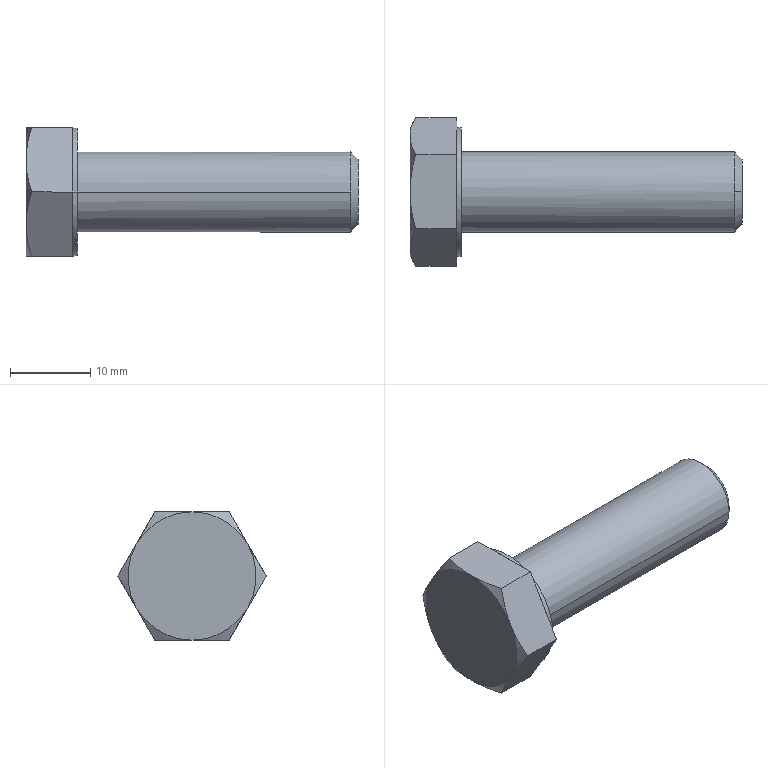Part | SolidWorks | features BaseBody 1 | 1 solid | 27 faces | box 41.4 x 18.475 x 16 mm | volume 4138 mm3 | plane 15 | cone 8 | cylinder 4 | commonest cylinder face diameters 10 x2 16 x2
STEP:
#1=CARTESIAN_POINT('',(0.,5.,0.));
#2=VERTEX_POINT('',#1);
#3=CARTESIAN_POINT('',(0.,-5.,0.));
#4=VERTEX_POINT('',#3);
#5=CARTESIAN_POINT('',(0.,0.,0.));
#6=DIRECTION('',(1.,0.,0.));
#7=DIRECTION('',(0.,1.,0.));
#8=AXIS2_PLACEMENT_3D('',#5,#6,#7);
#9=CIRCLE('',#8,5.);
#10=EDGE_CURVE('',#2,#4,#9,.T.);
#11=ORIENTED_EDGE('',*,*,#10,.T.);
#12=CARTESIAN_POINT('',(34.08,-5.,0.));
#13=VERTEX_POINT('',#12);
#14=CARTESIAN_POINT('',(19.75,-5.,0.));
#15=DIRECTION('',(1.,0.,0.));
#16=VECTOR('',#15,1000.);
#17=LINE('',#14,#16);
#18=EDGE_CURVE('',#4,#13,#17,.T.);
#19=ORIENTED_EDGE('',*,*,#18,.T.);
#20=CARTESIAN_POINT('',(34.08,0.,5.));
#21=VERTEX_POINT('',#20);
#22=CARTESIAN_POINT('',(34.08,0.,0.));
#23=DIRECTION('',(-1.,0.,0.));
#24=DIRECTION('',(0.,1.,0.));
#25=AXIS2_PLACEMENT_3D('',#22,#23,#24);
#26=CIRCLE('',#25,5.);
#27=EDGE_CURVE('',#13,#21,#26,.T.);
#28=ORIENTED_EDGE('',*,*,#27,.T.);
#29=CARTESIAN_POINT('',(34.08,5.,0.));
#30=VERTEX_POINT('',#29);
#31=CARTESIAN_POINT('',(34.08,0.,0.));
#32=DIRECTION('',(-1.,0.,0.));
#33=DIRECTION('',(0.,1.,0.));
#34=AXIS2_PLACEMENT_3D('',#31,#32,#33);
#35=CIRCLE('',#34,5.);
#36=EDGE_CURVE('',#21,#30,#35,.T.);
#37=ORIENTED_EDGE('',*,*,#36,.T.);
#38=CARTESIAN_POINT('',(19.75,5.,0.));
#39=DIRECTION('',(1.,0.,0.));
#40=VECTOR('',#39,1000.);
#41=LINE('',#38,#40);
#42=EDGE_CURVE('',#2,#30,#41,.T.);
#43=ORIENTED_EDGE('',*,*,#42,.F.);
#44=EDGE_LOOP('',(#11,#19,#28,#37,#43));
#45=FACE_OUTER_BOUND('',#44,.T.);
#46=CARTESIAN_POINT('',(19.75,0.,0.));
#47=DIRECTION('',(1.,0.,0.));
#48=DIRECTION('',(0.,1.,0.));
#49=AXIS2_PLACEMENT_3D('',#46,#47,#48);
#50=CYLINDRICAL_SURFACE('',#49,5.);
#51=ADVANCED_FACE('',(#45),#50,.T.);
#52=CARTESIAN_POINT('',(35.,0.,4.08));
#53=VERTEX_POINT('',#52);
#54=CARTESIAN_POINT('',(35.,0.,-4.08));
#55=VERTEX_POINT('',#54);
#56=CARTESIAN_POINT('',(35.,0.,0.));
#57=DIRECTION('',(-1.,0.,0.));
#58=DIRECTION('',(0.,0.,1.));
#59=AXIS2_PLACEMENT_3D('',#56,#57,#58);
#60=CIRCLE('',#59,4.08);
#61=EDGE_CURVE('',#53,#55,#60,.T.);
#62=ORIENTED_EDGE('',*,*,#61,.T.);
#63=CARTESIAN_POINT('',(34.08,0.,-5.));
#64=VERTEX_POINT('',#63);
#65=CARTESIAN_POINT('',(34.08,0.,-5.));
#66=DIRECTION('',(-0.7071,0.,-0.7071));
#67=VECTOR('',#66,1000.);
#68=LINE('',#65,#67);
#69=EDGE_CURVE('',#55,#64,#68,.T.);
#70=ORIENTED_EDGE('',*,*,#69,.T.);
#71=CARTESIAN_POINT('',(34.08,0.,0.));
#72=DIRECTION('',(-1.,0.,0.));
#73=DIRECTION('',(0.,1.,0.));
#74=AXIS2_PLACEMENT_3D('',#71,#72,#73);
#75=CIRCLE('',#74,5.);
#76=EDGE_CURVE('',#30,#64,#75,.T.);
#77=ORIENTED_EDGE('',*,*,#76,.F.);
#78=ORIENTED_EDGE('',*,*,#36,.F.);
#79=CARTESIAN_POINT('',(34.08,0.,5.));
#80=DIRECTION('',(-0.7071,0.,0.7071));
#81=VECTOR('',#80,1000.);
#82=LINE('',#79,#81);
#83=EDGE_CURVE('',#53,#21,#82,.T.);
#84=ORIENTED_EDGE('',*,*,#83,.F.);
#85=EDGE_LOOP('',(#62,#70,#77,#78,#84));
#86=FACE_OUTER_BOUND('',#85,.T.);
#87=CARTESIAN_POINT('',(34.08,0.,0.));
#88=DIRECTION('',(-1.,0.,0.));
#89=DIRECTION('',(0.,0.,1.));
#90=AXIS2_PLACEMENT_3D('',#87,#88,#89);
#91=CONICAL_SURFACE('',#90,5.,0.7853);
#92=ADVANCED_FACE('',(#86),#91,.T.);
#93=CARTESIAN_POINT('',(-0.6001,-6.928,4.));
#94=VERTEX_POINT('',#93);
#95=CARTESIAN_POINT('',(-0.6001,-8.,0.));
#96=VERTEX_POINT('',#95);
#97=CARTESIAN_POINT('',(-0.6001,0.,0.));
#98=DIRECTION('',(1.,0.,0.));
#99=DIRECTION('',(0.,1.,0.));
#100=AXIS2_PLACEMENT_3D('',#97,#98,#99);
#101=CIRCLE('',#100,8.);
#102=EDGE_CURVE('',#94,#96,#101,.T.);
#103=ORIENTED_EDGE('',*,*,#102,.T.);
#104=CARTESIAN_POINT('',(0.,-8.,0.));
#105=VERTEX_POINT('',#104);
#106=CARTESIAN_POINT('',(-0.3,-8.,0.));
#107=DIRECTION('',(1.,0.,0.));
#108=VECTOR('',#107,1000.);
#109=LINE('',#106,#108);
#110=EDGE_CURVE('',#96,#105,#109,.T.);
#111=ORIENTED_EDGE('',*,*,#110,.T.);
#112=CARTESIAN_POINT('',(0.,8.,0.));
#113=VERTEX_POINT('',#112);
#114=CARTESIAN_POINT('',(0.,0.,0.));
#115=DIRECTION('',(1.,0.,0.));
#116=DIRECTION('',(0.,1.,0.));
#117=AXIS2_PLACEMENT_3D('',#114,#115,#116);
#118=CIRCLE('',#117,8.);
#119=EDGE_CURVE('',#113,#105,#118,.T.);
#120=ORIENTED_EDGE('',*,*,#119,.F.);
#121=CARTESIAN_POINT('',(-0.6001,8.,0.));
#122=VERTEX_POINT('',#121);
#123=CARTESIAN_POINT('',(-0.3,8.,0.));
#124=DIRECTION('',(1.,0.,0.));
#125=VECTOR('',#124,1000.);
#126=LINE('',#123,#125);
#127=EDGE_CURVE('',#122,#113,#126,.T.);
#128=ORIENTED_EDGE('',*,*,#127,.F.);
#129=CARTESIAN_POINT('',(-0.6001,6.928,4.));
#130=VERTEX_POINT('',#129);
#131=CARTESIAN_POINT('',(-0.6001,0.,0.));
#132=DIRECTION('',(1.,0.,0.));
#133=DIRECTION('',(0.,1.,0.));
#134=AXIS2_PLACEMENT_3D('',#131,#132,#133);
#135=CIRCLE('',#134,8.);
#136=EDGE_CURVE('',#122,#130,#135,.T.);
#137=ORIENTED_EDGE('',*,*,#136,.T.);
#138=CARTESIAN_POINT('',(-0.6001,0.,8.));
#139=VERTEX_POINT('',#138);
#140=CARTESIAN_POINT('',(-0.6001,0.,0.));
#141=DIRECTION('',(1.,0.,0.));
#142=DIRECTION('',(0.,1.,0.));
#143=AXIS2_PLACEMENT_3D('',#140,#141,#142);
#144=CIRCLE('',#143,8.);
#145=EDGE_CURVE('',#130,#139,#144,.T.);
#146=ORIENTED_EDGE('',*,*,#145,.T.);
#147=CARTESIAN_POINT('',(-0.6001,0.,0.));
#148=DIRECTION('',(1.,0.,0.));
#149=DIRECTION('',(0.,1.,0.));
#150=AXIS2_PLACEMENT_3D('',#147,#148,#149);
#151=CIRCLE('',#150,8.);
#152=EDGE_CURVE('',#139,#94,#151,.T.);
#153=ORIENTED_EDGE('',*,*,#152,.T.);
#154=EDGE_LOOP('',(#103,#111,#120,#128,#137,#146,#153));
#155=FACE_OUTER_BOUND('',#154,.T.);
#156=CARTESIAN_POINT('',(-0.3,0.,0.));
#157=DIRECTION('',(1.,0.,0.));
#158=DIRECTION('',(0.,1.,0.));
#159=AXIS2_PLACEMENT_3D('',#156,#157,#158);
#160=CYLINDRICAL_SURFACE('',#159,8.);
#161=ADVANCED_FACE('',(#155),#160,.T.);
#162=ORIENTED_EDGE('',*,*,#18,.F.);
#163=CARTESIAN_POINT('',(0.,0.,0.));
#164=DIRECTION('',(1.,0.,0.));
#165=DIRECTION('',(0.,1.,0.));
#166=AXIS2_PLACEMENT_3D('',#163,#164,#165);
#167=CIRCLE('',#166,5.);
#168=EDGE_CURVE('',#4,#2,#167,.T.);
#169=ORIENTED_EDGE('',*,*,#168,.T.);
#170=ORIENTED_EDGE('',*,*,#42,.T.);
#171=ORIENTED_EDGE('',*,*,#76,.T.);
#172=CARTESIAN_POINT('',(34.08,0.,0.));
#173=DIRECTION('',(-1.,0.,0.));
#174=DIRECTION('',(0.,1.,0.));
#175=AXIS2_PLACEMENT_3D('',#172,#173,#174);
#176=CIRCLE('',#175,5.);
#177=EDGE_CURVE('',#64,#13,#176,.T.);
#178=ORIENTED_EDGE('',*,*,#177,.T.);
#179=EDGE_LOOP('',(#162,#169,#170,#171,#178));
#180=FACE_OUTER_BOUND('',#179,.T.);
#181=CARTESIAN_POINT('',(19.75,0.,0.));
#182=DIRECTION('',(1.,0.,0.));
#183=DIRECTION('',(0.,1.,0.));
#184=AXIS2_PLACEMENT_3D('',#181,#182,#183);
#185=CYLINDRICAL_SURFACE('',#184,5.);
#186=ADVANCED_FACE('',(#180),#185,.T.);
#187=ORIENTED_EDGE('',*,*,#69,.F.);
#188=CARTESIAN_POINT('',(35.,0.,0.));
#189=DIRECTION('',(-1.,0.,0.));
#190=DIRECTION('',(0.,0.,1.));
#191=AXIS2_PLACEMENT_3D('',#188,#189,#190);
#192=CIRCLE('',#191,4.08);
#193=EDGE_CURVE('',#55,#53,#192,.T.);
#194=ORIENTED_EDGE('',*,*,#193,.T.);
#195=ORIENTED_EDGE('',*,*,#83,.T.);
#196=ORIENTED_EDGE('',*,*,#27,.F.);
#197=ORIENTED_EDGE('',*,*,#177,.F.);
#198=EDGE_LOOP('',(#187,#194,#195,#196,#197));
#199=FACE_OUTER_BOUND('',#198,.T.);
#200=CARTESIAN_POINT('',(34.08,0.,0.));
#201=DIRECTION('',(-1.,0.,0.));
#202=DIRECTION('',(0.,0.,1.));
#203=AXIS2_PLACEMENT_3D('',#200,#201,#202);
#204=CONICAL_SURFACE('',#203,5.,0.7853);
#205=ADVANCED_FACE('',(#199),#204,.T.);
#206=ORIENTED_EDGE('',*,*,#10,.F.);
#207=ORIENTED_EDGE('',*,*,#168,.F.);
#208=EDGE_LOOP('',(#206,#207));
#209=FACE_BOUND('',#208,.T.);
#210=ORIENTED_EDGE('',*,*,#119,.T.);
#211=CARTESIAN_POINT('',(0.,0.,0.));
#212=DIRECTION('',(1.,0.,0.));
#213=DIRECTION('',(0.,1.,0.));
#214=AXIS2_PLACEMENT_3D('',#211,#212,#213);
#215=CIRCLE('',#214,8.);
#216=EDGE_CURVE('',#105,#113,#215,.T.);
#217=ORIENTED_EDGE('',*,*,#216,.T.);
#218=EDGE_LOOP('',(#210,#217));
#219=FACE_OUTER_BOUND('',#218,.T.);
#220=CARTESIAN_POINT('',(0.,6.5,0.));
#221=DIRECTION('',(1.,0.,0.));
#222=DIRECTION('',(0.,1.,0.));
#223=AXIS2_PLACEMENT_3D('',#220,#221,#222);
#224=PLANE('',#223);
#225=ADVANCED_FACE('',(#209,#219),#224,.T.);
#226=ORIENTED_EDGE('',*,*,#61,.F.);
#227=ORIENTED_EDGE('',*,*,#193,.F.);
#228=EDGE_LOOP('',(#226,#227));
#229=FACE_OUTER_BOUND('',#228,.T.);
#230=CARTESIAN_POINT('',(35.,2.5,0.));
#231=DIRECTION('',(1.,0.,0.));
#232=DIRECTION('',(0.,1.,0.));
#233=AXIS2_PLACEMENT_3D('',#230,#231,#232);
#234=PLANE('',#233);
#235=ADVANCED_FACE('',(#229),#234,.T.);
#236=ORIENTED_EDGE('',*,*,#110,.F.);
#237=CARTESIAN_POINT('',(-0.6001,-6.928,-4.));
#238=VERTEX_POINT('',#237);
#239=CARTESIAN_POINT('',(-0.6001,0.,0.));
#240=DIRECTION('',(1.,0.,0.));
#241=DIRECTION('',(0.,1.,0.));
#242=AXIS2_PLACEMENT_3D('',#239,#240,#241);
#243=CIRCLE('',#242,8.);
#244=EDGE_CURVE('',#96,#238,#243,.T.);
#245=ORIENTED_EDGE('',*,*,#244,.T.);
#246=CARTESIAN_POINT('',(-0.6001,0.,-8.));
#247=VERTEX_POINT('',#246);
#248=CARTESIAN_POINT('',(-0.6001,0.,0.));
#249=DIRECTION('',(1.,0.,0.));
#250=DIRECTION('',(0.,1.,0.));
#251=AXIS2_PLACEMENT_3D('',#248,#249,#250);
#252=CIRCLE('',#251,8.);
#253=EDGE_CURVE('',#238,#247,#252,.T.);
#254=ORIENTED_EDGE('',*,*,#253,.T.);
#255=CARTESIAN_POINT('',(-0.6001,6.928,-4.));
#256=VERTEX_POINT('',#255);
#257=CARTESIAN_POINT('',(-0.6001,0.,0.));
#258=DIRECTION('',(1.,0.,0.));
#259=DIRECTION('',(0.,1.,0.));
#260=AXIS2_PLACEMENT_3D('',#257,#258,#259);
#261=CIRCLE('',#260,8.);
#262=EDGE_CURVE('',#247,#256,#261,.T.);
#263=ORIENTED_EDGE('',*,*,#262,.T.);
#264=CARTESIAN_POINT('',(-0.6001,0.,0.));
#265=DIRECTION('',(1.,0.,0.));
#266=DIRECTION('',(0.,1.,0.));
#267=AXIS2_PLACEMENT_3D('',#264,#265,#266);
#268=CIRCLE('',#267,8.);
#269=EDGE_CURVE('',#256,#122,#268,.T.);
#270=ORIENTED_EDGE('',*,*,#269,.T.);
#271=ORIENTED_EDGE('',*,*,#127,.T.);
#272=ORIENTED_EDGE('',*,*,#216,.F.);
#273=EDGE_LOOP('',(#236,#245,#254,#263,#270,#271,#272));
#274=FACE_OUTER_BOUND('',#273,.T.);
#275=CARTESIAN_POINT('',(-0.3,0.,0.));
#276=DIRECTION('',(1.,0.,0.));
#277=DIRECTION('',(0.,1.,0.));
#278=AXIS2_PLACEMENT_3D('',#275,#276,#277);
#279=CYLINDRICAL_SURFACE('',#278,8.);
#280=ADVANCED_FACE('',(#274),#279,.T.);
#281=CARTESIAN_POINT('',(-0.6001,4.619,-8.));
#282=VERTEX_POINT('',#281);
#283=CARTESIAN_POINT('',(-0.6001,0.,-8.));
#284=DIRECTION('',(0.,1.,0.));
#285=VECTOR('',#284,1000.);
#286=LINE('',#283,#285);
#287=EDGE_CURVE('',#247,#282,#286,.T.);
#288=ORIENTED_EDGE('',*,*,#287,.T.);
#289=CARTESIAN_POINT('',(-0.6001,4.619,-8.));
#290=DIRECTION('',(0.,0.5,0.866));
#291=VECTOR('',#290,1000.);
#292=LINE('',#289,#291);
#293=EDGE_CURVE('',#282,#256,#292,.T.);
#294=ORIENTED_EDGE('',*,*,#293,.T.);
#295=ORIENTED_EDGE('',*,*,#262,.F.);
#296=EDGE_LOOP('',(#288,#294,#295));
#297=FACE_OUTER_BOUND('',#296,.T.);
#298=CARTESIAN_POINT('',(-0.6001,0.,0.));
#299=DIRECTION('',(1.,0.,0.));
#300=DIRECTION('',(0.,1.,0.));
#301=AXIS2_PLACEMENT_3D('',#298,#299,#300);
#302=PLANE('',#301);
#303=ADVANCED_FACE('',(#297),#302,.T.);
#304=CARTESIAN_POINT('',(-0.6001,-4.619,-8.));
#305=VERTEX_POINT('',#304);
#306=CARTESIAN_POINT('',(-0.6001,-6.928,-4.));
#307=DIRECTION('',(0.,0.5,-0.866));
#308=VECTOR('',#307,1000.);
#309=LINE('',#306,#308);
#310=EDGE_CURVE('',#238,#305,#309,.T.);
#311=ORIENTED_EDGE('',*,*,#310,.T.);
#312=CARTESIAN_POINT('',(-0.6001,0.,-8.));
#313=DIRECTION('',(0.,1.,0.));
#314=VECTOR('',#313,1000.);
#315=LINE('',#312,#314);
#316=EDGE_CURVE('',#305,#247,#315,.T.);
#317=ORIENTED_EDGE('',*,*,#316,.T.);
#318=ORIENTED_EDGE('',*,*,#253,.F.);
#319=EDGE_LOOP('',(#311,#317,#318));
#320=FACE_OUTER_BOUND('',#319,.T.);
#321=CARTESIAN_POINT('',(-0.6001,0.,0.));
#322=DIRECTION('',(1.,0.,0.));
#323=DIRECTION('',(0.,1.,0.));
#324=AXIS2_PLACEMENT_3D('',#321,#322,#323);
#325=PLANE('',#324);
#326=ADVANCED_FACE('',(#320),#325,.T.);
#327=CARTESIAN_POINT('',(-0.6001,-9.238,0.));
#328=VERTEX_POINT('',#327);
#329=CARTESIAN_POINT('',(-0.6001,-6.928,4.));
#330=DIRECTION('',(0.,-0.5,-0.866));
#331=VECTOR('',#330,1000.);
#332=LINE('',#329,#331);
#333=EDGE_CURVE('',#94,#328,#332,.T.);
#334=ORIENTED_EDGE('',*,*,#333,.T.);
#335=CARTESIAN_POINT('',(-0.6001,-9.238,0.));
#336=DIRECTION('',(0.,0.5,-0.866));
#337=VECTOR('',#336,1000.);
#338=LINE('',#335,#337);
#339=EDGE_CURVE('',#328,#238,#338,.T.);
#340=ORIENTED_EDGE('',*,*,#339,.T.);
#341=ORIENTED_EDGE('',*,*,#244,.F.);
#342=ORIENTED_EDGE('',*,*,#102,.F.);
#343=EDGE_LOOP('',(#334,#340,#341,#342));
#344=FACE_OUTER_BOUND('',#343,.T.);
#345=CARTESIAN_POINT('',(-0.6001,0.,0.));
#346=DIRECTION('',(1.,0.,0.));
#347=DIRECTION('',(0.,1.,0.));
#348=AXIS2_PLACEMENT_3D('',#345,#346,#347);
#349=PLANE('',#348);
#350=ADVANCED_FACE('',(#344),#349,.T.);
#351=CARTESIAN_POINT('',(-0.6001,-4.619,8.));
#352=VERTEX_POINT('',#351);
#353=CARTESIAN_POINT('',(-0.6001,0.,8.));
#354=DIRECTION('',(0.,-1.,0.));
#355=VECTOR('',#354,1000.);
#356=LINE('',#353,#355);
#357=EDGE_CURVE('',#139,#352,#356,.T.);
#358=ORIENTED_EDGE('',*,*,#357,.T.);
#359=CARTESIAN_POINT('',(-0.6001,-4.619,8.));
#360=DIRECTION('',(0.,-0.5,-0.866));
#361=VECTOR('',#360,1000.);
#362=LINE('',#359,#361);
#363=EDGE_CURVE('',#352,#94,#362,.T.);
#364=ORIENTED_EDGE('',*,*,#363,.T.);
#365=ORIENTED_EDGE('',*,*,#152,.F.);
#366=EDGE_LOOP('',(#358,#364,#365));
#367=FACE_OUTER_BOUND('',#366,.T.);
#368=CARTESIAN_POINT('',(-0.6001,0.,0.));
#369=DIRECTION('',(1.,0.,0.));
#370=DIRECTION('',(0.,1.,0.));
#371=AXIS2_PLACEMENT_3D('',#368,#369,#370);
#372=PLANE('',#371);
#373=ADVANCED_FACE('',(#367),#372,.T.);
#374=CARTESIAN_POINT('',(-0.6001,4.619,8.));
#375=VERTEX_POINT('',#374);
#376=CARTESIAN_POINT('',(-0.6001,6.928,4.));
#377=DIRECTION('',(0.,-0.5,0.866));
#378=VECTOR('',#377,1000.);
#379=LINE('',#376,#378);
#380=EDGE_CURVE('',#130,#375,#379,.T.);
#381=ORIENTED_EDGE('',*,*,#380,.T.);
#382=CARTESIAN_POINT('',(-0.6001,0.,8.));
#383=DIRECTION('',(0.,-1.,0.));
#384=VECTOR('',#383,1000.);
#385=LINE('',#382,#384);
#386=EDGE_CURVE('',#375,#139,#385,.T.);
#387=ORIENTED_EDGE('',*,*,#386,.T.);
#388=ORIENTED_EDGE('',*,*,#145,.F.);
#389=EDGE_LOOP('',(#381,#387,#388));
#390=FACE_OUTER_BOUND('',#389,.T.);
#391=CARTESIAN_POINT('',(-0.6001,0.,0.));
#392=DIRECTION('',(1.,0.,0.));
#393=DIRECTION('',(0.,1.,0.));
#394=AXIS2_PLACEMENT_3D('',#391,#392,#393);
#395=PLANE('',#394);
#396=ADVANCED_FACE('',(#390),#395,.T.);
#397=CARTESIAN_POINT('',(-0.6001,9.238,0.));
#398=VERTEX_POINT('',#397);
#399=CARTESIAN_POINT('',(-0.6001,6.928,-4.));
#400=DIRECTION('',(0.,0.5,0.866));
#401=VECTOR('',#400,1000.);
#402=LINE('',#399,#401);
#403=EDGE_CURVE('',#256,#398,#402,.T.);
#404=ORIENTED_EDGE('',*,*,#403,.T.);
#405=CARTESIAN_POINT('',(-0.6001,9.238,0.));
#406=DIRECTION('',(0.,-0.5,0.866));
#407=VECTOR('',#406,1000.);
#408=LINE('',#405,#407);
#409=EDGE_CURVE('',#398,#130,#408,.T.);
#410=ORIENTED_EDGE('',*,*,#409,.T.);
#411=ORIENTED_EDGE('',*,*,#136,.F.);
#412=ORIENTED_EDGE('',*,*,#269,.F.);
#413=EDGE_LOOP('',(#404,#410,#411,#412));
#414=FACE_OUTER_BOUND('',#413,.T.);
#415=CARTESIAN_POINT('',(-0.6001,0.,0.));
#416=DIRECTION('',(1.,0.,0.));
#417=DIRECTION('',(0.,1.,0.));
#418=AXIS2_PLACEMENT_3D('',#415,#416,#417);
#419=PLANE('',#418);
#420=ADVANCED_FACE('',(#414),#419,.T.);
#421=ORIENTED_EDGE('',*,*,#293,.F.);
#422=CARTESIAN_POINT('',(-5.686,4.619,-8.));
#423=VERTEX_POINT('',#422);
#424=CARTESIAN_POINT('',(-0.6001,4.619,-8.));
#425=DIRECTION('',(-1.,0.,0.));
#426=VECTOR('',#425,1000.);
#427=LINE('',#424,#426);
#428=EDGE_CURVE('',#282,#423,#427,.T.);
#429=ORIENTED_EDGE('',*,*,#428,.T.);
#430=CARTESIAN_POINT('',(-6.4,6.928,-4.));
#431=VERTEX_POINT('',#430);
#432=CARTESIAN_POINT('',(-5.686,4.619,-8.));
#433=CARTESIAN_POINT('',(-5.903,4.996,-7.347));
#434=CARTESIAN_POINT('',(-6.083,5.376,-6.688));
#435=CARTESIAN_POINT('',(-6.332,6.145,-5.356));
#436=CARTESIAN_POINT('',(-6.4,6.534,-4.683));
#437=CARTESIAN_POINT('',(-6.4,6.928,-4.));
#438=B_SPLINE_CURVE_WITH_KNOTS('',3,(#432,#433,#434,#435,#436,#437),.UNSPECIFIED.,.F.,.F.,(4,2,4),(0.,0.002337,0.004674),.UNSPECIFIED.);
#439=EDGE_CURVE('',#423,#431,#438,.T.);
#440=ORIENTED_EDGE('',*,*,#439,.T.);
#441=CARTESIAN_POINT('',(-5.686,9.238,0.));
#442=VERTEX_POINT('',#441);
#443=CARTESIAN_POINT('',(-6.4,6.928,-4.));
#444=CARTESIAN_POINT('',(-6.4,7.322,-3.317));
#445=CARTESIAN_POINT('',(-6.332,7.711,-2.644));
#446=CARTESIAN_POINT('',(-6.083,8.48,-1.312));
#447=CARTESIAN_POINT('',(-5.903,8.86,-0.6534));
#448=CARTESIAN_POINT('',(-5.686,9.238,0.));
#449=B_SPLINE_CURVE_WITH_KNOTS('',3,(#443,#444,#445,#446,#447,#448),.UNSPECIFIED.,.F.,.F.,(4,2,4),(0.,0.002337,0.004674),.UNSPECIFIED.);
#450=EDGE_CURVE('',#431,#442,#449,.T.);
#451=ORIENTED_EDGE('',*,*,#450,.T.);
#452=CARTESIAN_POINT('',(-0.6001,9.238,0.));
#453=DIRECTION('',(1.,0.,0.));
#454=VECTOR('',#453,1000.);
#455=LINE('',#452,#454);
#456=EDGE_CURVE('',#442,#398,#455,.T.);
#457=ORIENTED_EDGE('',*,*,#456,.T.);
#458=ORIENTED_EDGE('',*,*,#403,.F.);
#459=EDGE_LOOP('',(#421,#429,#440,#451,#457,#458));
#460=FACE_OUTER_BOUND('',#459,.T.);
#461=CARTESIAN_POINT('',(-0.6001,4.619,-8.));
#462=DIRECTION('',(0.,0.866,-0.5));
#463=DIRECTION('',(0.,0.5,0.866));
#464=AXIS2_PLACEMENT_3D('',#461,#462,#463);
#465=PLANE('',#464);
#466=ADVANCED_FACE('',(#460),#465,.T.);
#467=ORIENTED_EDGE('',*,*,#316,.F.);
#468=CARTESIAN_POINT('',(-5.686,-4.619,-8.));
#469=VERTEX_POINT('',#468);
#470=CARTESIAN_POINT('',(-0.6001,-4.619,-8.));
#471=DIRECTION('',(-1.,0.,0.));
#472=VECTOR('',#471,1000.);
#473=LINE('',#470,#472);
#474=EDGE_CURVE('',#305,#469,#473,.T.);
#475=ORIENTED_EDGE('',*,*,#474,.T.);
#476=CARTESIAN_POINT('',(-6.4,0.,-8.));
#477=VERTEX_POINT('',#476);
#478=CARTESIAN_POINT('',(-5.686,-4.619,-8.));
#479=CARTESIAN_POINT('',(-5.903,-3.864,-8.));
#480=CARTESIAN_POINT('',(-6.083,-3.104,-8.));
#481=CARTESIAN_POINT('',(-6.332,-1.566,-8.));
#482=CARTESIAN_POINT('',(-6.4,-0.7882,-8.));
#483=CARTESIAN_POINT('',(-6.4,0.,-8.));
#484=B_SPLINE_CURVE_WITH_KNOTS('',3,(#478,#479,#480,#481,#482,#483),.UNSPECIFIED.,.F.,.F.,(4,2,4),(0.,0.002337,0.004674),.UNSPECIFIED.);
#485=EDGE_CURVE('',#469,#477,#484,.T.);
#486=ORIENTED_EDGE('',*,*,#485,.T.);
#487=CARTESIAN_POINT('',(-6.4,0.,-8.));
#488=CARTESIAN_POINT('',(-6.4,0.7882,-8.));
#489=CARTESIAN_POINT('',(-6.332,1.566,-8.));
#490=CARTESIAN_POINT('',(-6.083,3.104,-8.));
#491=CARTESIAN_POINT('',(-5.903,3.864,-8.));
#492=CARTESIAN_POINT('',(-5.686,4.619,-8.));
#493=B_SPLINE_CURVE_WITH_KNOTS('',3,(#487,#488,#489,#490,#491,#492),.UNSPECIFIED.,.F.,.F.,(4,2,4),(0.,0.002337,0.004674),.UNSPECIFIED.);
#494=EDGE_CURVE('',#477,#423,#493,.T.);
#495=ORIENTED_EDGE('',*,*,#494,.T.);
#496=ORIENTED_EDGE('',*,*,#428,.F.);
#497=ORIENTED_EDGE('',*,*,#287,.F.);
#498=EDGE_LOOP('',(#467,#475,#486,#495,#496,#497));
#499=FACE_OUTER_BOUND('',#498,.T.);
#500=CARTESIAN_POINT('',(-0.6001,-4.619,-8.));
#501=DIRECTION('',(0.,0.,-1.));
#502=DIRECTION('',(0.,1.,0.));
#503=AXIS2_PLACEMENT_3D('',#500,#501,#502);
#504=PLANE('',#503);
#505=ADVANCED_FACE('',(#499),#504,.T.);
#506=CARTESIAN_POINT('',(-5.686,-9.238,0.));
#507=VERTEX_POINT('',#506);
#508=CARTESIAN_POINT('',(-0.6001,-9.238,0.));
#509=DIRECTION('',(-1.,0.,0.));
#510=VECTOR('',#509,1000.);
#511=LINE('',#508,#510);
#512=EDGE_CURVE('',#328,#507,#511,.T.);
#513=ORIENTED_EDGE('',*,*,#512,.T.);
#514=CARTESIAN_POINT('',(-6.4,-6.928,-4.));
#515=VERTEX_POINT('',#514);
#516=CARTESIAN_POINT('',(-5.686,-9.238,0.));
#517=CARTESIAN_POINT('',(-5.903,-8.86,-0.6534));
#518=CARTESIAN_POINT('',(-6.083,-8.48,-1.312));
#519=CARTESIAN_POINT('',(-6.332,-7.711,-2.644));
#520=CARTESIAN_POINT('',(-6.4,-7.322,-3.317));
#521=CARTESIAN_POINT('',(-6.4,-6.928,-4.));
#522=B_SPLINE_CURVE_WITH_KNOTS('',3,(#516,#517,#518,#519,#520,#521),.UNSPECIFIED.,.F.,.F.,(4,2,4),(0.,0.002337,0.004674),.UNSPECIFIED.);
#523=EDGE_CURVE('',#507,#515,#522,.T.);
#524=ORIENTED_EDGE('',*,*,#523,.T.);
#525=CARTESIAN_POINT('',(-6.4,-6.928,-4.));
#526=CARTESIAN_POINT('',(-6.4,-6.534,-4.683));
#527=CARTESIAN_POINT('',(-6.332,-6.145,-5.356));
#528=CARTESIAN_POINT('',(-6.083,-5.376,-6.688));
#529=CARTESIAN_POINT('',(-5.903,-4.996,-7.347));
#530=CARTESIAN_POINT('',(-5.686,-4.619,-8.));
#531=B_SPLINE_CURVE_WITH_KNOTS('',3,(#525,#526,#527,#528,#529,#530),.UNSPECIFIED.,.F.,.F.,(4,2,4),(0.,0.002337,0.004674),.UNSPECIFIED.);
#532=EDGE_CURVE('',#515,#469,#531,.T.);
#533=ORIENTED_EDGE('',*,*,#532,.T.);
#534=ORIENTED_EDGE('',*,*,#474,.F.);
#535=ORIENTED_EDGE('',*,*,#310,.F.);
#536=ORIENTED_EDGE('',*,*,#339,.F.);
#537=EDGE_LOOP('',(#513,#524,#533,#534,#535,#536));
#538=FACE_OUTER_BOUND('',#537,.T.);
#539=CARTESIAN_POINT('',(-0.6001,-9.238,0.));
#540=DIRECTION('',(0.,-0.866,-0.5));
#541=DIRECTION('',(0.,0.5,-0.866));
#542=AXIS2_PLACEMENT_3D('',#539,#540,#541);
#543=PLANE('',#542);
#544=ADVANCED_FACE('',(#538),#543,.T.);
#545=CARTESIAN_POINT('',(-5.686,-4.619,8.));
#546=VERTEX_POINT('',#545);
#547=CARTESIAN_POINT('',(-0.6001,-4.619,8.));
#548=DIRECTION('',(-1.,0.,0.));
#549=VECTOR('',#548,1000.);
#550=LINE('',#547,#549);
#551=EDGE_CURVE('',#352,#546,#550,.T.);
#552=ORIENTED_EDGE('',*,*,#551,.T.);
#553=CARTESIAN_POINT('',(-6.4,-6.928,4.));
#554=VERTEX_POINT('',#553);
#555=CARTESIAN_POINT('',(-5.686,-4.619,8.));
#556=CARTESIAN_POINT('',(-5.903,-4.996,7.347));
#557=CARTESIAN_POINT('',(-6.083,-5.376,6.688));
#558=CARTESIAN_POINT('',(-6.332,-6.145,5.356));
#559=CARTESIAN_POINT('',(-6.4,-6.534,4.683));
#560=CARTESIAN_POINT('',(-6.4,-6.928,4.));
#561=B_SPLINE_CURVE_WITH_KNOTS('',3,(#555,#556,#557,#558,#559,#560),.UNSPECIFIED.,.F.,.F.,(4,2,4),(0.,0.002337,0.004674),.UNSPECIFIED.);
#562=EDGE_CURVE('',#546,#554,#561,.T.);
#563=ORIENTED_EDGE('',*,*,#562,.T.);
#564=CARTESIAN_POINT('',(-6.4,-6.928,4.));
#565=CARTESIAN_POINT('',(-6.4,-7.322,3.317));
#566=CARTESIAN_POINT('',(-6.332,-7.711,2.644));
#567=CARTESIAN_POINT('',(-6.083,-8.48,1.312));
#568=CARTESIAN_POINT('',(-5.903,-8.86,0.6534));
#569=CARTESIAN_POINT('',(-5.686,-9.238,0.));
#570=B_SPLINE_CURVE_WITH_KNOTS('',3,(#564,#565,#566,#567,#568,#569),.UNSPECIFIED.,.F.,.F.,(4,2,4),(0.,0.002337,0.004674),.UNSPECIFIED.);
#571=EDGE_CURVE('',#554,#507,#570,.T.);
#572=ORIENTED_EDGE('',*,*,#571,.T.);
#573=ORIENTED_EDGE('',*,*,#512,.F.);
#574=ORIENTED_EDGE('',*,*,#333,.F.);
#575=ORIENTED_EDGE('',*,*,#363,.F.);
#576=EDGE_LOOP('',(#552,#563,#572,#573,#574,#575));
#577=FACE_OUTER_BOUND('',#576,.T.);
#578=CARTESIAN_POINT('',(-0.6001,-4.619,8.));
#579=DIRECTION('',(0.,-0.866,0.5));
#580=DIRECTION('',(0.,-0.5,-0.866));
#581=AXIS2_PLACEMENT_3D('',#578,#579,#580);
#582=PLANE('',#581);
#583=ADVANCED_FACE('',(#577),#582,.T.);
#584=CARTESIAN_POINT('',(-5.686,4.619,8.));
#585=VERTEX_POINT('',#584);
#586=CARTESIAN_POINT('',(-0.6001,4.619,8.));
#587=DIRECTION('',(-1.,0.,0.));
#588=VECTOR('',#587,1000.);
#589=LINE('',#586,#588);
#590=EDGE_CURVE('',#375,#585,#589,.T.);
#591=ORIENTED_EDGE('',*,*,#590,.T.);
#592=CARTESIAN_POINT('',(-6.4,0.,8.));
#593=VERTEX_POINT('',#592);
#594=CARTESIAN_POINT('',(-5.686,4.619,8.));
#595=CARTESIAN_POINT('',(-5.903,3.864,8.));
#596=CARTESIAN_POINT('',(-6.083,3.104,8.));
#597=CARTESIAN_POINT('',(-6.332,1.566,8.));
#598=CARTESIAN_POINT('',(-6.4,0.7882,8.));
#599=CARTESIAN_POINT('',(-6.4,0.,8.));
#600=B_SPLINE_CURVE_WITH_KNOTS('',3,(#594,#595,#596,#597,#598,#599),.UNSPECIFIED.,.F.,.F.,(4,2,4),(0.,0.002337,0.004674),.UNSPECIFIED.);
#601=EDGE_CURVE('',#585,#593,#600,.T.);
#602=ORIENTED_EDGE('',*,*,#601,.T.);
#603=CARTESIAN_POINT('',(-6.4,0.,8.));
#604=CARTESIAN_POINT('',(-6.4,-0.7882,8.));
#605=CARTESIAN_POINT('',(-6.332,-1.566,8.));
#606=CARTESIAN_POINT('',(-6.083,-3.104,8.));
#607=CARTESIAN_POINT('',(-5.903,-3.864,8.));
#608=CARTESIAN_POINT('',(-5.686,-4.619,8.));
#609=B_SPLINE_CURVE_WITH_KNOTS('',3,(#603,#604,#605,#606,#607,#608),.UNSPECIFIED.,.F.,.F.,(4,2,4),(0.,0.002337,0.004674),.UNSPECIFIED.);
#610=EDGE_CURVE('',#593,#546,#609,.T.);
#611=ORIENTED_EDGE('',*,*,#610,.T.);
#612=ORIENTED_EDGE('',*,*,#551,.F.);
#613=ORIENTED_EDGE('',*,*,#357,.F.);
#614=ORIENTED_EDGE('',*,*,#386,.F.);
#615=EDGE_LOOP('',(#591,#602,#611,#612,#613,#614));
#616=FACE_OUTER_BOUND('',#615,.T.);
#617=CARTESIAN_POINT('',(-0.6001,4.619,8.));
#618=DIRECTION('',(0.,0.,1.));
#619=DIRECTION('',(0.,-1.,0.));
#620=AXIS2_PLACEMENT_3D('',#617,#618,#619);
#621=PLANE('',#620);
#622=ADVANCED_FACE('',(#616),#621,.T.);
#623=ORIENTED_EDGE('',*,*,#409,.F.);
#624=ORIENTED_EDGE('',*,*,#456,.F.);
#625=CARTESIAN_POINT('',(-6.4,6.928,4.));
#626=VERTEX_POINT('',#625);
#627=CARTESIAN_POINT('',(-5.686,9.238,0.));
#628=CARTESIAN_POINT('',(-5.903,8.86,0.6534));
#629=CARTESIAN_POINT('',(-6.083,8.48,1.312));
#630=CARTESIAN_POINT('',(-6.332,7.711,2.644));
#631=CARTESIAN_POINT('',(-6.4,7.322,3.317));
#632=CARTESIAN_POINT('',(-6.4,6.928,4.));
#633=B_SPLINE_CURVE_WITH_KNOTS('',3,(#627,#628,#629,#630,#631,#632),.UNSPECIFIED.,.F.,.F.,(4,2,4),(0.,0.002337,0.004674),.UNSPECIFIED.);
#634=EDGE_CURVE('',#442,#626,#633,.T.);
#635=ORIENTED_EDGE('',*,*,#634,.T.);
#636=CARTESIAN_POINT('',(-6.4,6.928,4.));
#637=CARTESIAN_POINT('',(-6.4,6.534,4.683));
#638=CARTESIAN_POINT('',(-6.332,6.145,5.356));
#639=CARTESIAN_POINT('',(-6.083,5.376,6.688));
#640=CARTESIAN_POINT('',(-5.903,4.996,7.347));
#641=CARTESIAN_POINT('',(-5.686,4.619,8.));
#642=B_SPLINE_CURVE_WITH_KNOTS('',3,(#636,#637,#638,#639,#640,#641),.UNSPECIFIED.,.F.,.F.,(4,2,4),(0.,0.002337,0.004674),.UNSPECIFIED.);
#643=EDGE_CURVE('',#626,#585,#642,.T.);
#644=ORIENTED_EDGE('',*,*,#643,.T.);
#645=ORIENTED_EDGE('',*,*,#590,.F.);
#646=ORIENTED_EDGE('',*,*,#380,.F.);
#647=EDGE_LOOP('',(#623,#624,#635,#644,#645,#646));
#648=FACE_OUTER_BOUND('',#647,.T.);
#649=CARTESIAN_POINT('',(-0.6001,9.238,0.));
#650=DIRECTION('',(0.,0.866,0.5));
#651=DIRECTION('',(0.,-0.5,0.866));
#652=AXIS2_PLACEMENT_3D('',#649,#650,#651);
#653=PLANE('',#652);
#654=ADVANCED_FACE('',(#648),#653,.T.);
#655=CARTESIAN_POINT('',(-6.4,0.,0.));
#656=DIRECTION('',(1.,0.,0.));
#657=DIRECTION('',(0.,0.,-1.));
#658=AXIS2_PLACEMENT_3D('',#655,#656,#657);
#659=CIRCLE('',#658,8.);
#660=EDGE_CURVE('',#431,#626,#659,.T.);
#661=ORIENTED_EDGE('',*,*,#660,.T.);
#662=ORIENTED_EDGE('',*,*,#634,.F.);
#663=ORIENTED_EDGE('',*,*,#450,.F.);
#664=EDGE_LOOP('',(#661,#662,#663));
#665=FACE_OUTER_BOUND('',#664,.T.);
#666=CARTESIAN_POINT('',(-5.681,0.,0.));
#667=DIRECTION('',(1.,0.,0.));
#668=DIRECTION('',(0.,0.,-1.));
#669=AXIS2_PLACEMENT_3D('',#666,#667,#668);
#670=CONICAL_SURFACE('',#669,9.245,1.047);
#671=ADVANCED_FACE('',(#665),#670,.T.);
#672=CARTESIAN_POINT('',(-6.4,0.,0.));
#673=DIRECTION('',(1.,0.,0.));
#674=DIRECTION('',(0.,0.,-1.));
#675=AXIS2_PLACEMENT_3D('',#672,#673,#674);
#676=CIRCLE('',#675,8.);
#677=EDGE_CURVE('',#477,#431,#676,.T.);
#678=ORIENTED_EDGE('',*,*,#677,.T.);
#679=ORIENTED_EDGE('',*,*,#439,.F.);
#680=ORIENTED_EDGE('',*,*,#494,.F.);
#681=EDGE_LOOP('',(#678,#679,#680));
#682=FACE_OUTER_BOUND('',#681,.T.);
#683=CARTESIAN_POINT('',(-5.681,0.,0.));
#684=DIRECTION('',(1.,0.,0.));
#685=DIRECTION('',(0.,0.,-1.));
#686=AXIS2_PLACEMENT_3D('',#683,#684,#685);
#687=CONICAL_SURFACE('',#686,9.245,1.047);
#688=ADVANCED_FACE('',(#682),#687,.T.);
#689=ORIENTED_EDGE('',*,*,#532,.F.);
#690=CARTESIAN_POINT('',(-6.4,0.,0.));
#691=DIRECTION('',(1.,0.,0.));
#692=DIRECTION('',(0.,0.,-1.));
#693=AXIS2_PLACEMENT_3D('',#690,#691,#692);
#694=CIRCLE('',#693,8.);
#695=EDGE_CURVE('',#515,#477,#694,.T.);
#696=ORIENTED_EDGE('',*,*,#695,.T.);
#697=ORIENTED_EDGE('',*,*,#485,.F.);
#698=EDGE_LOOP('',(#689,#696,#697));
#699=FACE_OUTER_BOUND('',#698,.T.);
#700=CARTESIAN_POINT('',(-5.681,0.,0.));
#701=DIRECTION('',(1.,0.,0.));
#702=DIRECTION('',(0.,0.,-1.));
#703=AXIS2_PLACEMENT_3D('',#700,#701,#702);
#704=CONICAL_SURFACE('',#703,9.245,1.047);
#705=ADVANCED_FACE('',(#699),#704,.T.);
#706=ORIENTED_EDGE('',*,*,#571,.F.);
#707=CARTESIAN_POINT('',(-6.4,0.,0.));
#708=DIRECTION('',(1.,0.,0.));
#709=DIRECTION('',(0.,0.,-1.));
#710=AXIS2_PLACEMENT_3D('',#707,#708,#709);
#711=CIRCLE('',#710,8.);
#712=EDGE_CURVE('',#554,#515,#711,.T.);
#713=ORIENTED_EDGE('',*,*,#712,.T.);
#714=ORIENTED_EDGE('',*,*,#523,.F.);
#715=EDGE_LOOP('',(#706,#713,#714));
#716=FACE_OUTER_BOUND('',#715,.T.);
#717=CARTESIAN_POINT('',(-5.681,0.,0.));
#718=DIRECTION('',(1.,0.,0.));
#719=DIRECTION('',(0.,0.,-1.));
#720=AXIS2_PLACEMENT_3D('',#717,#718,#719);
#721=CONICAL_SURFACE('',#720,9.245,1.047);
#722=ADVANCED_FACE('',(#716),#721,.T.);
#723=ORIENTED_EDGE('',*,*,#610,.F.);
#724=CARTESIAN_POINT('',(-6.4,0.,0.));
#725=DIRECTION('',(1.,0.,0.));
#726=DIRECTION('',(0.,0.,-1.));
#727=AXIS2_PLACEMENT_3D('',#724,#725,#726);
#728=CIRCLE('',#727,8.);
#729=EDGE_CURVE('',#593,#554,#728,.T.);
#730=ORIENTED_EDGE('',*,*,#729,.T.);
#731=ORIENTED_EDGE('',*,*,#562,.F.);
#732=EDGE_LOOP('',(#723,#730,#731));
#733=FACE_OUTER_BOUND('',#732,.T.);
#734=CARTESIAN_POINT('',(-5.681,0.,0.));
#735=DIRECTION('',(1.,0.,0.));
#736=DIRECTION('',(0.,0.,-1.));
#737=AXIS2_PLACEMENT_3D('',#734,#735,#736);
#738=CONICAL_SURFACE('',#737,9.245,1.047);
#739=ADVANCED_FACE('',(#733),#738,.T.);
#740=CARTESIAN_POINT('',(-6.4,0.,0.));
#741=DIRECTION('',(1.,0.,0.));
#742=DIRECTION('',(0.,0.,-1.));
#743=AXIS2_PLACEMENT_3D('',#740,#741,#742);
#744=CIRCLE('',#743,8.);
#745=EDGE_CURVE('',#626,#593,#744,.T.);
#746=ORIENTED_EDGE('',*,*,#745,.T.);
#747=ORIENTED_EDGE('',*,*,#601,.F.);
#748=ORIENTED_EDGE('',*,*,#643,.F.);
#749=EDGE_LOOP('',(#746,#747,#748));
#750=FACE_OUTER_BOUND('',#749,.T.);
#751=CARTESIAN_POINT('',(-5.681,0.,0.));
#752=DIRECTION('',(1.,0.,0.));
#753=DIRECTION('',(0.,0.,-1.));
#754=AXIS2_PLACEMENT_3D('',#751,#752,#753);
#755=CONICAL_SURFACE('',#754,9.245,1.047);
#756=ADVANCED_FACE('',(#750),#755,.T.);
#757=ORIENTED_EDGE('',*,*,#660,.F.);
#758=ORIENTED_EDGE('',*,*,#677,.F.);
#759=ORIENTED_EDGE('',*,*,#695,.F.);
#760=ORIENTED_EDGE('',*,*,#712,.F.);
#761=ORIENTED_EDGE('',*,*,#729,.F.);
#762=ORIENTED_EDGE('',*,*,#745,.F.);
#763=EDGE_LOOP('',(#757,#758,#759,#760,#761,#762));
#764=FACE_OUTER_BOUND('',#763,.T.);
#765=CARTESIAN_POINT('',(-6.4,0.,0.));
#766=DIRECTION('',(1.,0.,0.));
#767=DIRECTION('',(0.,1.,0.));
#768=AXIS2_PLACEMENT_3D('',#765,#766,#767);
#769=PLANE('',#768);
#770=ADVANCED_FACE('',(#764),#769,.F.);
#771=CLOSED_SHELL('',(#51,#92,#161,#186,#205,#225,#235,#280,#303,#326,#350,#373,#396,#420,#466,#505,#544,#583,#622,#654,#671,#688,#705,#722,#739,#756,#770));
#772=MANIFOLD_SOLID_BREP('',#771);
#773=CARTESIAN_POINT('',(0.,0.,0.));
#774=DIRECTION('',(0.,0.,1.));
#775=DIRECTION('',(1.,0.,0.));
#776=AXIS2_PLACEMENT_3D('',#773,#774,#775);
#777=(LENGTH_UNIT()NAMED_UNIT(*)SI_UNIT(.MILLI.,.METRE.));
#778=UNCERTAINTY_MEASURE_WITH_UNIT(LENGTH_MEASURE(0.00001),#777,'','');
#779=(NAMED_UNIT(*)PLANE_ANGLE_UNIT()SI_UNIT($,.RADIAN.));
#780=(NAMED_UNIT(*)SI_UNIT($,.STERADIAN.)SOLID_ANGLE_UNIT());
#781=(GEOMETRIC_REPRESENTATION_CONTEXT(3)GLOBAL_UNCERTAINTY_ASSIGNED_CONTEXT((#778))GLOBAL_UNIT_ASSIGNED_CONTEXT((#777,#779,#780))REPRESENTATION_CONTEXT('',''));
#782=ADVANCED_BREP_SHAPE_REPRESENTATION('',(#772,#776),#781);